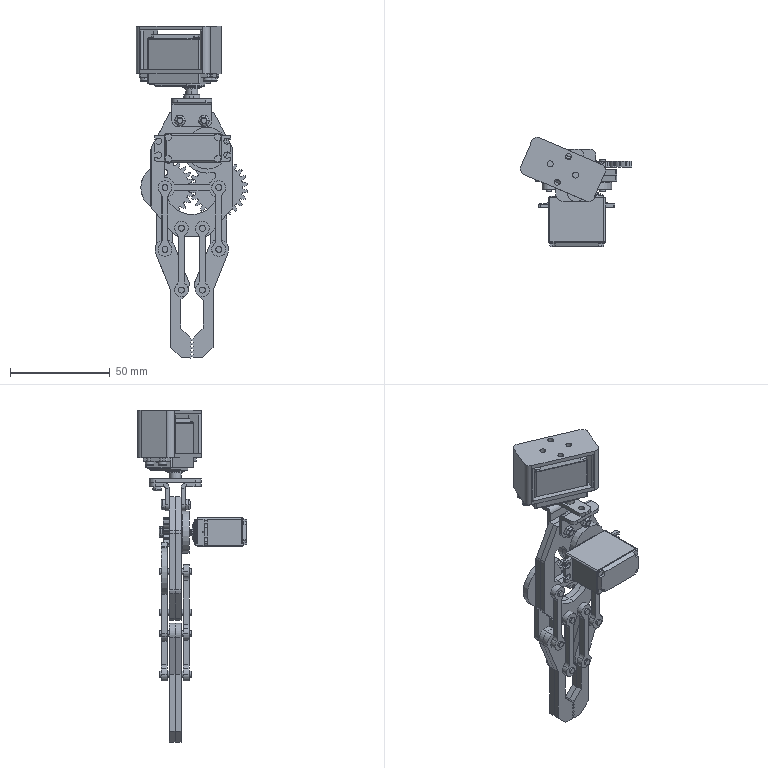Part | SolidWorks | features CompositeCurve 4, AEMSimFeature 1 | 42 solids | 1715 faces | box 55.908 x 54.775 x 166.65 mm | volume 52779 mm3 | cylinder 943 | plane 694 | spline 36 | torus 32 | sphere 8 | cone 2 | commonest cylinder face diameters 3 x294 10.8 x127 4.361 x92 6 x54 1.4 x48 2.86 x38